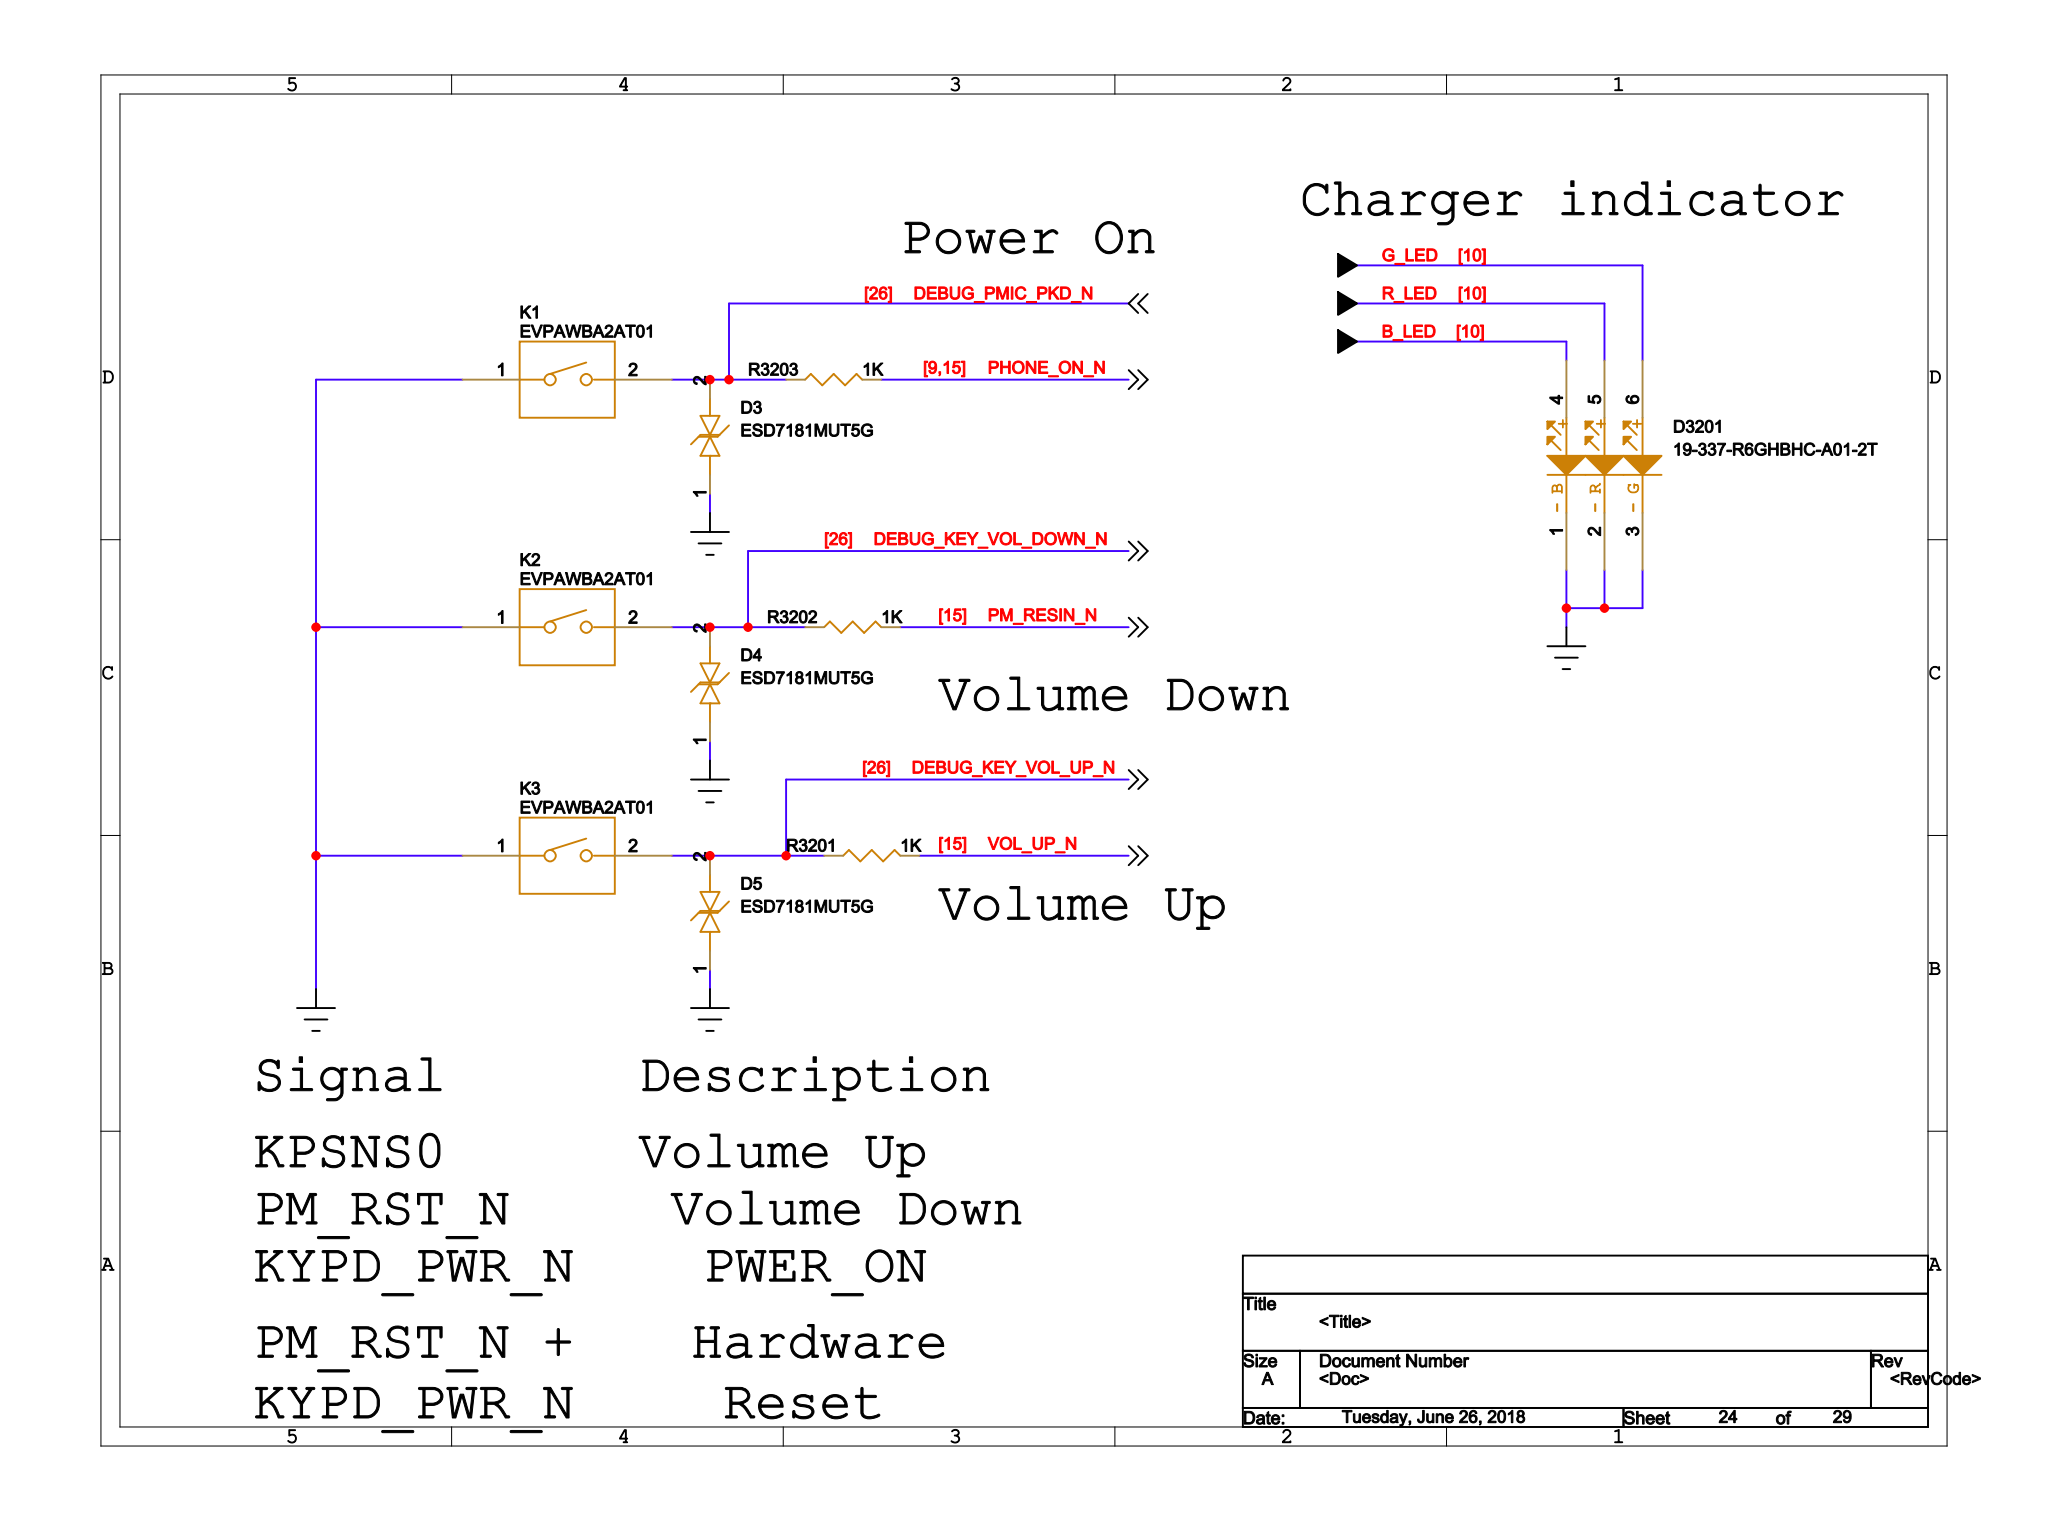Circuit board | Cadence Allegro | 802 parts | 566 nets | one sheet of the schematic
Parts on this sheet (reference | value | footprint):
D3 | ESD7181MUT5G | X3DFN2_0P62X0P32_0P43_0P355
D4 | ESD7181MUT5G | X3DFN2_0P62X0P32_0P43_0P355
D5 | ESD7181MUT5G | X3DFN2_0P62X0P32_0P43_0P355
D3201 | 19-337-R6GHBHC-A01-2T | 19-337-R6GHBHC-A01-2T
K1 | EVPAWBA2AT01 | KEY_EVPAWBA2AT01
K2 | EVPAWBA2AT01 | KEY_EVPAWBA2AT01
K3 | EVPAWBA2AT01 | KEY_EVPAWBA2AT01
R3201 | 1K | R0201
R3202 | 1K | R0201
R3203 | 1K | R0201
Nets of these parts (net: part-pin ...):
GND: D3-1 D4-1 D5-1 D3201-1 D3201-2 D3201-3 K1-1 K2-1 K3-1
DEBUG_PMIC_PKD_N: D3-2 K1-2 R3203-1
DEBUG_KEY_VOL_DOWN_N: D4-2 K2-2 R3202-1
DEBUG_KEY_VOL_UP_N: D5-2 K3-2 R3201-1
B_LED: D3201-4
G_LED: D3201-6
R_LED: D3201-5
VOL_UP_N: R3201-2
PM_RESIN_N: R3202-2
PHONE_ON_N: R3203-2